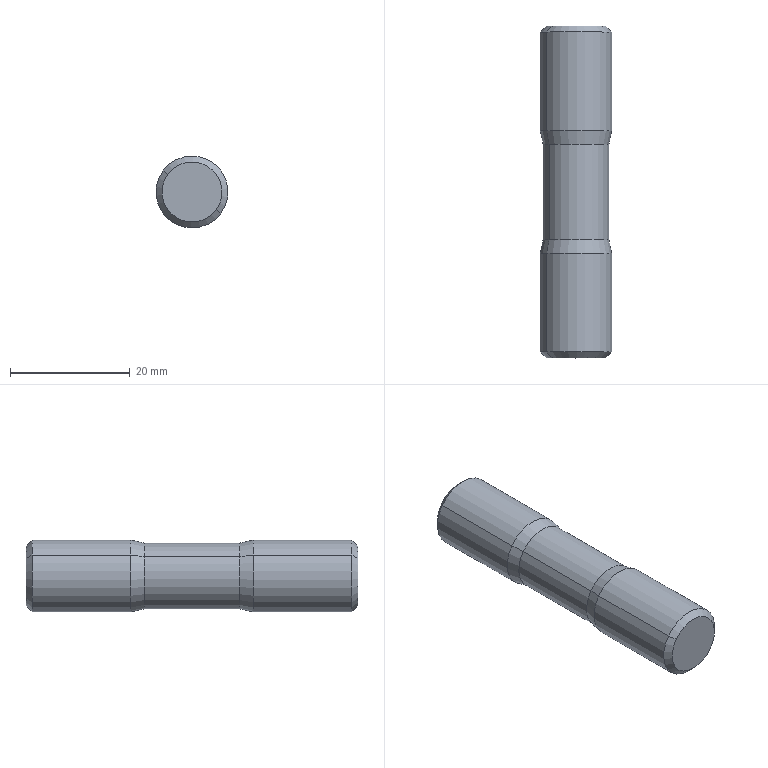Part | SolidWorks | features BaseBody 1 | 1 solid | 16 faces | box 12 x 55.4 x 12 mm | volume 5900 mm3 | cone 8 | cylinder 6 | plane 2 | commonest cylinder face diameters 12 x4 11 x2
STEP:
#1=CARTESIAN_POINT('',(26.559,139.,21.33));
#2=VERTEX_POINT('',#1);
#3=CARTESIAN_POINT('',(18.441,139.,27.17));
#4=VERTEX_POINT('',#3);
#5=CARTESIAN_POINT('',(22.5,139.,24.25));
#6=DIRECTION('',(0.,-1.,0.));
#7=DIRECTION('',(0.8118,0.,-0.584));
#8=AXIS2_PLACEMENT_3D('',#5,#6,#7);
#9=CIRCLE('',#8,5.);
#10=EDGE_CURVE('',#2,#4,#9,.T.);
#11=ORIENTED_EDGE('',*,*,#10,.F.);
#12=CARTESIAN_POINT('',(27.371,140.,20.746));
#13=VERTEX_POINT('',#12);
#14=CARTESIAN_POINT('',(26.559,139.,21.33));
#15=DIRECTION('',(0.574,0.7071,-0.4129));
#16=VECTOR('',#15,1000.);
#17=LINE('',#14,#16);
#18=EDGE_CURVE('',#2,#13,#17,.T.);
#19=ORIENTED_EDGE('',*,*,#18,.T.);
#20=CARTESIAN_POINT('',(17.629,140.,27.754));
#21=VERTEX_POINT('',#20);
#22=CARTESIAN_POINT('',(22.5,140.,24.25));
#23=DIRECTION('',(0.,1.,0.));
#24=DIRECTION('',(0.8118,0.,-0.584));
#25=AXIS2_PLACEMENT_3D('',#22,#23,#24);
#26=CIRCLE('',#25,6.);
#27=EDGE_CURVE('',#21,#13,#26,.T.);
#28=ORIENTED_EDGE('',*,*,#27,.F.);
#29=CARTESIAN_POINT('',(18.441,139.,27.17));
#30=DIRECTION('',(-0.574,0.7071,0.4129));
#31=VECTOR('',#30,1000.);
#32=LINE('',#29,#31);
#33=EDGE_CURVE('',#4,#21,#32,.T.);
#34=ORIENTED_EDGE('',*,*,#33,.F.);
#35=EDGE_LOOP('',(#11,#19,#28,#34));
#36=FACE_OUTER_BOUND('',#35,.T.);
#37=CARTESIAN_POINT('',(22.5,139.,24.25));
#38=DIRECTION('',(0.,1.,0.));
#39=DIRECTION('',(-0.8118,0.,0.584));
#40=AXIS2_PLACEMENT_3D('',#37,#38,#39);
#41=CONICAL_SURFACE('',#40,5.,0.7854);
#42=ADVANCED_FACE('',(#36),#41,.T.);
#43=CARTESIAN_POINT('',(18.441,194.4,27.17));
#44=VERTEX_POINT('',#43);
#45=CARTESIAN_POINT('',(26.559,194.4,21.33));
#46=VERTEX_POINT('',#45);
#47=CARTESIAN_POINT('',(22.5,194.4,24.25));
#48=DIRECTION('',(0.,1.,0.));
#49=DIRECTION('',(0.8118,0.,-0.584));
#50=AXIS2_PLACEMENT_3D('',#47,#48,#49);
#51=CIRCLE('',#50,5.);
#52=EDGE_CURVE('',#44,#46,#51,.T.);
#53=ORIENTED_EDGE('',*,*,#52,.F.);
#54=CARTESIAN_POINT('',(17.629,193.4,27.754));
#55=VERTEX_POINT('',#54);
#56=CARTESIAN_POINT('',(17.629,193.4,27.754));
#57=DIRECTION('',(-0.574,-0.7071,0.4129));
#58=VECTOR('',#57,1000.);
#59=LINE('',#56,#58);
#60=EDGE_CURVE('',#44,#55,#59,.T.);
#61=ORIENTED_EDGE('',*,*,#60,.T.);
#62=CARTESIAN_POINT('',(27.371,193.4,20.746));
#63=VERTEX_POINT('',#62);
#64=CARTESIAN_POINT('',(22.5,193.4,24.25));
#65=DIRECTION('',(0.,-1.,0.));
#66=DIRECTION('',(0.8118,0.,-0.584));
#67=AXIS2_PLACEMENT_3D('',#64,#65,#66);
#68=CIRCLE('',#67,6.);
#69=EDGE_CURVE('',#63,#55,#68,.T.);
#70=ORIENTED_EDGE('',*,*,#69,.F.);
#71=CARTESIAN_POINT('',(27.371,193.4,20.746));
#72=DIRECTION('',(0.574,-0.7071,-0.4129));
#73=VECTOR('',#72,1000.);
#74=LINE('',#71,#73);
#75=EDGE_CURVE('',#46,#63,#74,.T.);
#76=ORIENTED_EDGE('',*,*,#75,.F.);
#77=EDGE_LOOP('',(#53,#61,#70,#76));
#78=FACE_OUTER_BOUND('',#77,.T.);
#79=CARTESIAN_POINT('',(22.5,193.4,24.25));
#80=DIRECTION('',(0.,-1.,0.));
#81=DIRECTION('',(0.8118,0.,-0.584));
#82=AXIS2_PLACEMENT_3D('',#79,#80,#81);
#83=CONICAL_SURFACE('',#82,6.,0.7854);
#84=ADVANCED_FACE('',(#78),#83,.T.);
#85=ORIENTED_EDGE('',*,*,#69,.T.);
#86=CARTESIAN_POINT('',(17.629,176.95,27.754));
#87=VERTEX_POINT('',#86);
#88=CARTESIAN_POINT('',(17.629,194.4,27.754));
#89=DIRECTION('',(0.,-1.,0.));
#90=VECTOR('',#89,1000.);
#91=LINE('',#88,#90);
#92=EDGE_CURVE('',#55,#87,#91,.T.);
#93=ORIENTED_EDGE('',*,*,#92,.T.);
#94=CARTESIAN_POINT('',(27.371,176.95,20.746));
#95=VERTEX_POINT('',#94);
#96=CARTESIAN_POINT('',(22.5,176.95,24.25));
#97=DIRECTION('',(0.,-1.,0.));
#98=DIRECTION('',(0.8118,0.,-0.584));
#99=AXIS2_PLACEMENT_3D('',#96,#97,#98);
#100=CIRCLE('',#99,6.);
#101=EDGE_CURVE('',#95,#87,#100,.T.);
#102=ORIENTED_EDGE('',*,*,#101,.F.);
#103=CARTESIAN_POINT('',(27.371,194.4,20.746));
#104=DIRECTION('',(0.,-1.,0.));
#105=VECTOR('',#104,1000.);
#106=LINE('',#103,#105);
#107=EDGE_CURVE('',#63,#95,#106,.T.);
#108=ORIENTED_EDGE('',*,*,#107,.F.);
#109=EDGE_LOOP('',(#85,#93,#102,#108));
#110=FACE_OUTER_BOUND('',#109,.T.);
#111=CARTESIAN_POINT('',(22.5,194.4,24.25));
#112=DIRECTION('',(0.,-1.,0.));
#113=DIRECTION('',(0.8118,0.,-0.584));
#114=AXIS2_PLACEMENT_3D('',#111,#112,#113);
#115=CYLINDRICAL_SURFACE('',#114,6.);
#116=ADVANCED_FACE('',(#110),#115,.T.);
#117=CARTESIAN_POINT('',(26.965,174.7,21.038));
#118=VERTEX_POINT('',#117);
#119=CARTESIAN_POINT('',(18.035,174.7,27.462));
#120=VERTEX_POINT('',#119);
#121=CARTESIAN_POINT('',(22.5,174.7,24.25));
#122=DIRECTION('',(0.,-1.,0.));
#123=DIRECTION('',(0.8118,0.,-0.584));
#124=AXIS2_PLACEMENT_3D('',#121,#122,#123);
#125=CIRCLE('',#124,5.5);
#126=EDGE_CURVE('',#118,#120,#125,.T.);
#127=ORIENTED_EDGE('',*,*,#126,.F.);
#128=CARTESIAN_POINT('',(26.965,174.7,21.038));
#129=DIRECTION('',(0.1761,0.9762,-0.1267));
#130=VECTOR('',#129,1000.);
#131=LINE('',#128,#130);
#132=EDGE_CURVE('',#118,#95,#131,.T.);
#133=ORIENTED_EDGE('',*,*,#132,.T.);
#134=ORIENTED_EDGE('',*,*,#101,.T.);
#135=CARTESIAN_POINT('',(18.035,174.7,27.462));
#136=DIRECTION('',(-0.1761,0.9762,0.1267));
#137=VECTOR('',#136,1000.);
#138=LINE('',#135,#137);
#139=EDGE_CURVE('',#120,#87,#138,.T.);
#140=ORIENTED_EDGE('',*,*,#139,.F.);
#141=EDGE_LOOP('',(#127,#133,#134,#140));
#142=FACE_OUTER_BOUND('',#141,.T.);
#143=CARTESIAN_POINT('',(22.5,174.7,24.25));
#144=DIRECTION('',(0.,1.,0.));
#145=DIRECTION('',(-0.8118,0.,0.584));
#146=AXIS2_PLACEMENT_3D('',#143,#144,#145);
#147=CONICAL_SURFACE('',#146,5.5,0.2187);
#148=ADVANCED_FACE('',(#142),#147,.T.);
#149=ORIENTED_EDGE('',*,*,#126,.T.);
#150=CARTESIAN_POINT('',(18.035,158.7,27.462));
#151=VERTEX_POINT('',#150);
#152=CARTESIAN_POINT('',(18.035,138.005,27.462));
#153=DIRECTION('',(0.,-1.,0.));
#154=VECTOR('',#153,1000.);
#155=LINE('',#152,#154);
#156=EDGE_CURVE('',#120,#151,#155,.T.);
#157=ORIENTED_EDGE('',*,*,#156,.T.);
#158=CARTESIAN_POINT('',(26.965,158.7,21.038));
#159=VERTEX_POINT('',#158);
#160=CARTESIAN_POINT('',(22.5,158.7,24.25));
#161=DIRECTION('',(0.,-1.,0.));
#162=DIRECTION('',(0.8118,0.,-0.584));
#163=AXIS2_PLACEMENT_3D('',#160,#161,#162);
#164=CIRCLE('',#163,5.5);
#165=EDGE_CURVE('',#159,#151,#164,.T.);
#166=ORIENTED_EDGE('',*,*,#165,.F.);
#167=CARTESIAN_POINT('',(26.965,138.005,21.038));
#168=DIRECTION('',(0.,-1.,0.));
#169=VECTOR('',#168,1000.);
#170=LINE('',#167,#169);
#171=EDGE_CURVE('',#118,#159,#170,.T.);
#172=ORIENTED_EDGE('',*,*,#171,.F.);
#173=EDGE_LOOP('',(#149,#157,#166,#172));
#174=FACE_OUTER_BOUND('',#173,.T.);
#175=CARTESIAN_POINT('',(22.5,138.005,24.25));
#176=DIRECTION('',(0.,-1.,0.));
#177=DIRECTION('',(0.8118,0.,-0.584));
#178=AXIS2_PLACEMENT_3D('',#175,#176,#177);
#179=CYLINDRICAL_SURFACE('',#178,5.5);
#180=ADVANCED_FACE('',(#174),#179,.T.);
#181=ORIENTED_EDGE('',*,*,#165,.T.);
#182=CARTESIAN_POINT('',(17.629,156.45,27.754));
#183=VERTEX_POINT('',#182);
#184=CARTESIAN_POINT('',(17.629,156.45,27.754));
#185=DIRECTION('',(-0.1761,-0.9762,0.1267));
#186=VECTOR('',#185,1000.);
#187=LINE('',#184,#186);
#188=EDGE_CURVE('',#151,#183,#187,.T.);
#189=ORIENTED_EDGE('',*,*,#188,.T.);
#190=CARTESIAN_POINT('',(27.371,156.45,20.746));
#191=VERTEX_POINT('',#190);
#192=CARTESIAN_POINT('',(22.5,156.45,24.25));
#193=DIRECTION('',(0.,-1.,0.));
#194=DIRECTION('',(0.8118,0.,-0.584));
#195=AXIS2_PLACEMENT_3D('',#192,#193,#194);
#196=CIRCLE('',#195,6.);
#197=EDGE_CURVE('',#191,#183,#196,.T.);
#198=ORIENTED_EDGE('',*,*,#197,.F.);
#199=CARTESIAN_POINT('',(27.371,156.45,20.746));
#200=DIRECTION('',(0.1761,-0.9762,-0.1267));
#201=VECTOR('',#200,1000.);
#202=LINE('',#199,#201);
#203=EDGE_CURVE('',#159,#191,#202,.T.);
#204=ORIENTED_EDGE('',*,*,#203,.F.);
#205=EDGE_LOOP('',(#181,#189,#198,#204));
#206=FACE_OUTER_BOUND('',#205,.T.);
#207=CARTESIAN_POINT('',(22.5,156.45,24.25));
#208=DIRECTION('',(0.,-1.,0.));
#209=DIRECTION('',(0.8118,0.,-0.584));
#210=AXIS2_PLACEMENT_3D('',#207,#208,#209);
#211=CONICAL_SURFACE('',#210,6.,0.2187);
#212=ADVANCED_FACE('',(#206),#211,.T.);
#213=ORIENTED_EDGE('',*,*,#197,.T.);
#214=CARTESIAN_POINT('',(17.629,194.4,27.754));
#215=DIRECTION('',(0.,-1.,0.));
#216=VECTOR('',#215,1000.);
#217=LINE('',#214,#216);
#218=EDGE_CURVE('',#183,#21,#217,.T.);
#219=ORIENTED_EDGE('',*,*,#218,.T.);
#220=ORIENTED_EDGE('',*,*,#27,.T.);
#221=CARTESIAN_POINT('',(27.371,194.4,20.746));
#222=DIRECTION('',(0.,-1.,0.));
#223=VECTOR('',#222,1000.);
#224=LINE('',#221,#223);
#225=EDGE_CURVE('',#191,#13,#224,.T.);
#226=ORIENTED_EDGE('',*,*,#225,.F.);
#227=EDGE_LOOP('',(#213,#219,#220,#226));
#228=FACE_OUTER_BOUND('',#227,.T.);
#229=CARTESIAN_POINT('',(22.5,194.4,24.25));
#230=DIRECTION('',(0.,-1.,0.));
#231=DIRECTION('',(0.8118,0.,-0.584));
#232=AXIS2_PLACEMENT_3D('',#229,#230,#231);
#233=CYLINDRICAL_SURFACE('',#232,6.);
#234=ADVANCED_FACE('',(#228),#233,.T.);
#235=ORIENTED_EDGE('',*,*,#218,.F.);
#236=CARTESIAN_POINT('',(22.5,156.45,24.25));
#237=DIRECTION('',(0.,-1.,0.));
#238=DIRECTION('',(0.8118,0.,-0.584));
#239=AXIS2_PLACEMENT_3D('',#236,#237,#238);
#240=CIRCLE('',#239,6.);
#241=EDGE_CURVE('',#183,#191,#240,.T.);
#242=ORIENTED_EDGE('',*,*,#241,.T.);
#243=ORIENTED_EDGE('',*,*,#225,.T.);
#244=CARTESIAN_POINT('',(22.5,140.,24.25));
#245=DIRECTION('',(0.,1.,0.));
#246=DIRECTION('',(0.8118,0.,-0.584));
#247=AXIS2_PLACEMENT_3D('',#244,#245,#246);
#248=CIRCLE('',#247,6.);
#249=EDGE_CURVE('',#13,#21,#248,.T.);
#250=ORIENTED_EDGE('',*,*,#249,.T.);
#251=EDGE_LOOP('',(#235,#242,#243,#250));
#252=FACE_OUTER_BOUND('',#251,.T.);
#253=CARTESIAN_POINT('',(22.5,194.4,24.25));
#254=DIRECTION('',(0.,-1.,0.));
#255=DIRECTION('',(0.8118,0.,-0.584));
#256=AXIS2_PLACEMENT_3D('',#253,#254,#255);
#257=CYLINDRICAL_SURFACE('',#256,6.);
#258=ADVANCED_FACE('',(#252),#257,.T.);
#259=CARTESIAN_POINT('',(22.5,139.,24.25));
#260=DIRECTION('',(0.,-1.,0.));
#261=DIRECTION('',(0.8118,0.,-0.584));
#262=AXIS2_PLACEMENT_3D('',#259,#260,#261);
#263=CIRCLE('',#262,5.);
#264=EDGE_CURVE('',#4,#2,#263,.T.);
#265=ORIENTED_EDGE('',*,*,#264,.T.);
#266=ORIENTED_EDGE('',*,*,#10,.T.);
#267=EDGE_LOOP('',(#265,#266));
#268=FACE_OUTER_BOUND('',#267,.T.);
#269=CARTESIAN_POINT('',(22.5,139.,24.25));
#270=DIRECTION('',(0.,-1.,0.));
#271=DIRECTION('',(0.8118,0.,-0.584));
#272=AXIS2_PLACEMENT_3D('',#269,#270,#271);
#273=PLANE('',#272);
#274=ADVANCED_FACE('',(#268),#273,.T.);
#275=ORIENTED_EDGE('',*,*,#188,.F.);
#276=CARTESIAN_POINT('',(22.5,158.7,24.25));
#277=DIRECTION('',(0.,-1.,0.));
#278=DIRECTION('',(0.8118,0.,-0.584));
#279=AXIS2_PLACEMENT_3D('',#276,#277,#278);
#280=CIRCLE('',#279,5.5);
#281=EDGE_CURVE('',#151,#159,#280,.T.);
#282=ORIENTED_EDGE('',*,*,#281,.T.);
#283=ORIENTED_EDGE('',*,*,#203,.T.);
#284=ORIENTED_EDGE('',*,*,#241,.F.);
#285=EDGE_LOOP('',(#275,#282,#283,#284));
#286=FACE_OUTER_BOUND('',#285,.T.);
#287=CARTESIAN_POINT('',(22.5,156.45,24.25));
#288=DIRECTION('',(0.,-1.,0.));
#289=DIRECTION('',(0.8118,0.,-0.584));
#290=AXIS2_PLACEMENT_3D('',#287,#288,#289);
#291=CONICAL_SURFACE('',#290,6.,0.2187);
#292=ADVANCED_FACE('',(#286),#291,.T.);
#293=ORIENTED_EDGE('',*,*,#156,.F.);
#294=CARTESIAN_POINT('',(22.5,174.7,24.25));
#295=DIRECTION('',(0.,-1.,0.));
#296=DIRECTION('',(0.8118,0.,-0.584));
#297=AXIS2_PLACEMENT_3D('',#294,#295,#296);
#298=CIRCLE('',#297,5.5);
#299=EDGE_CURVE('',#120,#118,#298,.T.);
#300=ORIENTED_EDGE('',*,*,#299,.T.);
#301=ORIENTED_EDGE('',*,*,#171,.T.);
#302=ORIENTED_EDGE('',*,*,#281,.F.);
#303=EDGE_LOOP('',(#293,#300,#301,#302));
#304=FACE_OUTER_BOUND('',#303,.T.);
#305=CARTESIAN_POINT('',(22.5,138.005,24.25));
#306=DIRECTION('',(0.,-1.,0.));
#307=DIRECTION('',(0.8118,0.,-0.584));
#308=AXIS2_PLACEMENT_3D('',#305,#306,#307);
#309=CYLINDRICAL_SURFACE('',#308,5.5);
#310=ADVANCED_FACE('',(#304),#309,.T.);
#311=ORIENTED_EDGE('',*,*,#132,.F.);
#312=ORIENTED_EDGE('',*,*,#299,.F.);
#313=ORIENTED_EDGE('',*,*,#139,.T.);
#314=CARTESIAN_POINT('',(22.5,176.95,24.25));
#315=DIRECTION('',(0.,-1.,0.));
#316=DIRECTION('',(0.8118,0.,-0.584));
#317=AXIS2_PLACEMENT_3D('',#314,#315,#316);
#318=CIRCLE('',#317,6.);
#319=EDGE_CURVE('',#87,#95,#318,.T.);
#320=ORIENTED_EDGE('',*,*,#319,.T.);
#321=EDGE_LOOP('',(#311,#312,#313,#320));
#322=FACE_OUTER_BOUND('',#321,.T.);
#323=CARTESIAN_POINT('',(22.5,174.7,24.25));
#324=DIRECTION('',(0.,1.,0.));
#325=DIRECTION('',(-0.8118,0.,0.584));
#326=AXIS2_PLACEMENT_3D('',#323,#324,#325);
#327=CONICAL_SURFACE('',#326,5.5,0.2187);
#328=ADVANCED_FACE('',(#322),#327,.T.);
#329=CARTESIAN_POINT('',(22.5,194.4,24.25));
#330=DIRECTION('',(0.,1.,0.));
#331=DIRECTION('',(0.8118,0.,-0.584));
#332=AXIS2_PLACEMENT_3D('',#329,#330,#331);
#333=CIRCLE('',#332,5.);
#334=EDGE_CURVE('',#46,#44,#333,.T.);
#335=ORIENTED_EDGE('',*,*,#334,.T.);
#336=ORIENTED_EDGE('',*,*,#52,.T.);
#337=EDGE_LOOP('',(#335,#336));
#338=FACE_OUTER_BOUND('',#337,.T.);
#339=CARTESIAN_POINT('',(22.5,194.4,24.25));
#340=DIRECTION('',(0.,-1.,0.));
#341=DIRECTION('',(0.8118,0.,-0.584));
#342=AXIS2_PLACEMENT_3D('',#339,#340,#341);
#343=PLANE('',#342);
#344=ADVANCED_FACE('',(#338),#343,.F.);
#345=ORIENTED_EDGE('',*,*,#92,.F.);
#346=CARTESIAN_POINT('',(22.5,193.4,24.25));
#347=DIRECTION('',(0.,-1.,0.));
#348=DIRECTION('',(0.8118,0.,-0.584));
#349=AXIS2_PLACEMENT_3D('',#346,#347,#348);
#350=CIRCLE('',#349,6.);
#351=EDGE_CURVE('',#55,#63,#350,.T.);
#352=ORIENTED_EDGE('',*,*,#351,.T.);
#353=ORIENTED_EDGE('',*,*,#107,.T.);
#354=ORIENTED_EDGE('',*,*,#319,.F.);
#355=EDGE_LOOP('',(#345,#352,#353,#354));
#356=FACE_OUTER_BOUND('',#355,.T.);
#357=CARTESIAN_POINT('',(22.5,194.4,24.25));
#358=DIRECTION('',(0.,-1.,0.));
#359=DIRECTION('',(0.8118,0.,-0.584));
#360=AXIS2_PLACEMENT_3D('',#357,#358,#359);
#361=CYLINDRICAL_SURFACE('',#360,6.);
#362=ADVANCED_FACE('',(#356),#361,.T.);
#363=ORIENTED_EDGE('',*,*,#60,.F.);
#364=ORIENTED_EDGE('',*,*,#334,.F.);
#365=ORIENTED_EDGE('',*,*,#75,.T.);
#366=ORIENTED_EDGE('',*,*,#351,.F.);
#367=EDGE_LOOP('',(#363,#364,#365,#366));
#368=FACE_OUTER_BOUND('',#367,.T.);
#369=CARTESIAN_POINT('',(22.5,193.4,24.25));
#370=DIRECTION('',(0.,-1.,0.));
#371=DIRECTION('',(0.8118,0.,-0.584));
#372=AXIS2_PLACEMENT_3D('',#369,#370,#371);
#373=CONICAL_SURFACE('',#372,6.,0.7854);
#374=ADVANCED_FACE('',(#368),#373,.T.);
#375=ORIENTED_EDGE('',*,*,#18,.F.);
#376=ORIENTED_EDGE('',*,*,#264,.F.);
#377=ORIENTED_EDGE('',*,*,#33,.T.);
#378=ORIENTED_EDGE('',*,*,#249,.F.);
#379=EDGE_LOOP('',(#375,#376,#377,#378));
#380=FACE_OUTER_BOUND('',#379,.T.);
#381=CARTESIAN_POINT('',(22.5,139.,24.25));
#382=DIRECTION('',(0.,1.,0.));
#383=DIRECTION('',(-0.8118,0.,0.584));
#384=AXIS2_PLACEMENT_3D('',#381,#382,#383);
#385=CONICAL_SURFACE('',#384,5.,0.7854);
#386=ADVANCED_FACE('',(#380),#385,.T.);
#387=CLOSED_SHELL('',(#42,#84,#116,#148,#180,#212,#234,#258,#274,#292,#310,#328,#344,#362,#374,#386));
#388=MANIFOLD_SOLID_BREP('',#387);
#389=CARTESIAN_POINT('',(0.,0.,0.));
#390=DIRECTION('',(0.,0.,1.));
#391=DIRECTION('',(1.,0.,0.));
#392=AXIS2_PLACEMENT_3D('',#389,#390,#391);
#393=(LENGTH_UNIT()NAMED_UNIT(*)SI_UNIT(.MILLI.,.METRE.));
#394=UNCERTAINTY_MEASURE_WITH_UNIT(LENGTH_MEASURE(0.00001),#393,'','');
#395=(NAMED_UNIT(*)PLANE_ANGLE_UNIT()SI_UNIT($,.RADIAN.));
#396=(NAMED_UNIT(*)SI_UNIT($,.STERADIAN.)SOLID_ANGLE_UNIT());
#397=(GEOMETRIC_REPRESENTATION_CONTEXT(3)GLOBAL_UNCERTAINTY_ASSIGNED_CONTEXT((#394))GLOBAL_UNIT_ASSIGNED_CONTEXT((#393,#395,#396))REPRESENTATION_CONTEXT('',''));
#398=ADVANCED_BREP_SHAPE_REPRESENTATION('',(#388,#392),#397);